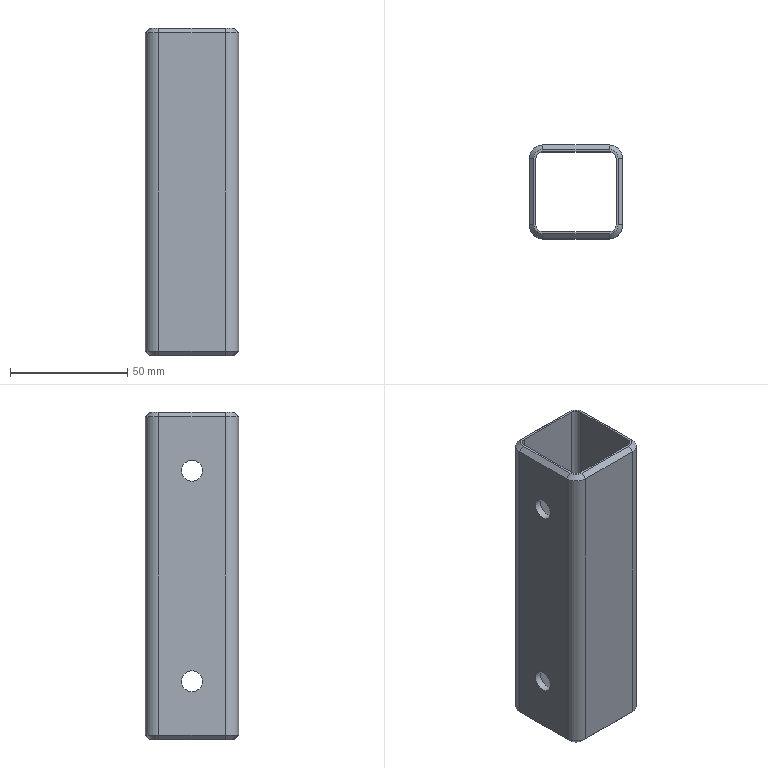Part | STEP file | DIN 59 410 - PPTM_02 | 1 solid | 38 faces | box 40 x 40 x 140 mm | volume 55897 mm3 | plane 18 | cylinder 12 | cone 8 | commonest cylinder face diameters 5.8 x4 9 x4 11.6 x4